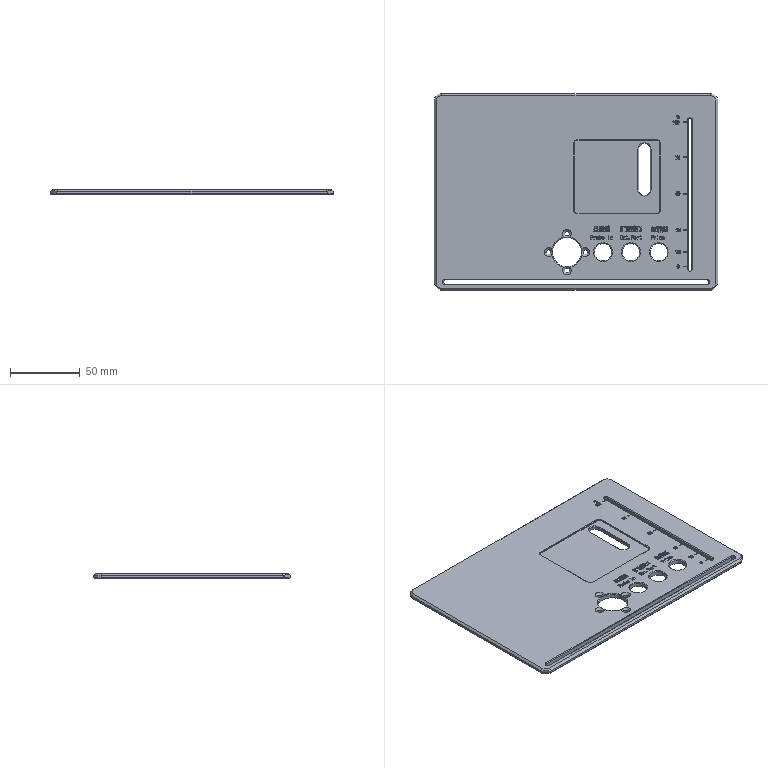Part | SolidWorks | features BaseBody 1 | 1 solid | 1088 faces | box 204 x 141.5 x 3.5 mm | volume 90078 mm3 | plane 567 | spline 443 | cone 41 | cylinder 37 | commonest cylinder face diameters 3.4 x8 12.5 x6 1 x4 4 x4 3.1 x3 2.5 x2